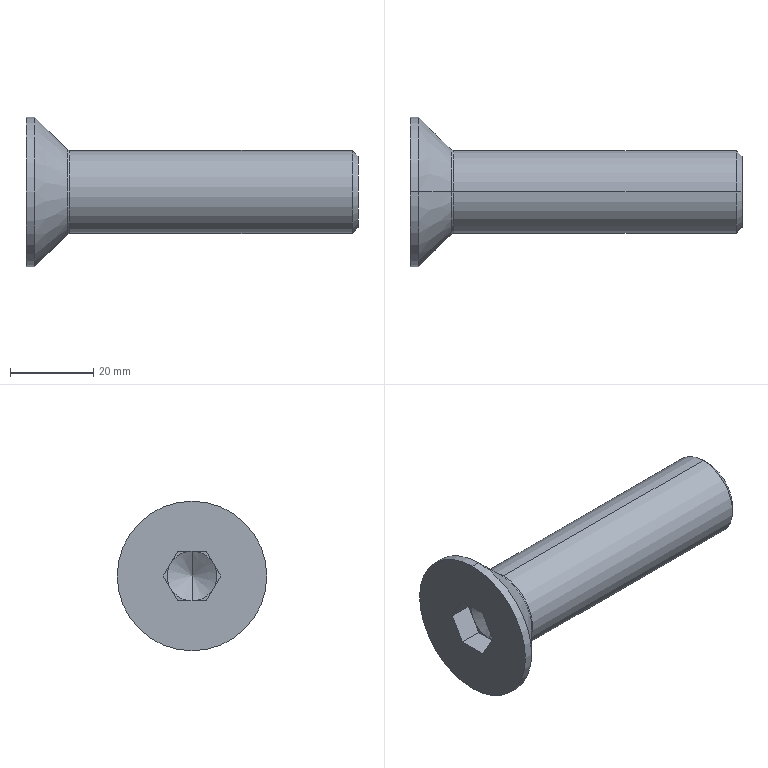Part | SolidWorks | features BaseBody 1 | 1 solid | 26 faces | box 80 x 36.05 x 36.05 mm | volume 28321 mm3 | plane 14 | cone 6 | cylinder 4 | spline 2 | commonest cylinder face diameters 20 x2 36.05 x2
STEP:
#1=CARTESIAN_POINT('',(10.491,0.,-10.));
#2=VERTEX_POINT('',#1);
#3=CARTESIAN_POINT('',(10.491,0.,10.));
#4=VERTEX_POINT('',#3);
#5=CARTESIAN_POINT('',(10.491,0.,0.));
#6=DIRECTION('',(1.,0.,0.));
#7=DIRECTION('',(0.,0.,1.));
#8=AXIS2_PLACEMENT_3D('',#5,#6,#7);
#9=CIRCLE('',#8,10.);
#10=EDGE_CURVE('',#2,#4,#9,.T.);
#11=ORIENTED_EDGE('',*,*,#10,.F.);
#12=CARTESIAN_POINT('',(9.926,0.,-10.234));
#13=VERTEX_POINT('',#12);
#14=CARTESIAN_POINT('',(10.491,0.,-10.8));
#15=DIRECTION('',(0.,-1.,0.));
#16=DIRECTION('',(0.,0.,-1.));
#17=AXIS2_PLACEMENT_3D('',#14,#15,#16);
#18=CIRCLE('',#17,0.8);
#19=EDGE_CURVE('',#2,#13,#18,.T.);
#20=ORIENTED_EDGE('',*,*,#19,.T.);
#21=CARTESIAN_POINT('',(9.926,0.,10.234));
#22=VERTEX_POINT('',#21);
#23=CARTESIAN_POINT('',(9.926,0.,0.));
#24=DIRECTION('',(-1.,0.,0.));
#25=DIRECTION('',(0.,0.,1.));
#26=AXIS2_PLACEMENT_3D('',#23,#24,#25);
#27=CIRCLE('',#26,10.234);
#28=EDGE_CURVE('',#22,#13,#27,.T.);
#29=ORIENTED_EDGE('',*,*,#28,.F.);
#30=CARTESIAN_POINT('',(10.491,0.,10.8));
#31=DIRECTION('',(0.,1.,0.));
#32=DIRECTION('',(0.,0.,1.));
#33=AXIS2_PLACEMENT_3D('',#30,#31,#32);
#34=CIRCLE('',#33,0.8);
#35=EDGE_CURVE('',#4,#22,#34,.T.);
#36=ORIENTED_EDGE('',*,*,#35,.F.);
#37=EDGE_LOOP('',(#11,#20,#29,#36));
#38=FACE_OUTER_BOUND('',#37,.T.);
#39=CARTESIAN_POINT('',(10.491,0.,10.));
#40=CARTESIAN_POINT('',(10.491,20.,10.));
#41=CARTESIAN_POINT('',(10.491,20.,-10.));
#42=CARTESIAN_POINT('',(10.491,0.,-10.));
#43=CARTESIAN_POINT('',(10.276,0.,10.));
#44=CARTESIAN_POINT('',(10.276,20.,10.));
#45=CARTESIAN_POINT('',(10.276,20.,-10.));
#46=CARTESIAN_POINT('',(10.276,0.,-10.));
#47=CARTESIAN_POINT('',(10.078,0.,10.082));
#48=CARTESIAN_POINT('',(10.078,20.165,10.082));
#49=CARTESIAN_POINT('',(10.078,20.165,-10.082));
#50=CARTESIAN_POINT('',(10.078,0.,-10.082));
#51=CARTESIAN_POINT('',(9.926,0.,10.234));
#52=CARTESIAN_POINT('',(9.926,20.469,10.234));
#53=CARTESIAN_POINT('',(9.926,20.469,-10.234));
#54=CARTESIAN_POINT('',(9.926,0.,-10.234));
#55=(BOUNDED_SURFACE()B_SPLINE_SURFACE(3,3,((#39,#40,#41,#42),(#43,#44,#45,#46),(#47,#48,#49,#50),(#51,#52,#53,#54)),.UNSPECIFIED.,.F.,.F.,.F.)B_SPLINE_SURFACE_WITH_KNOTS((4,4),(4,4),(0.,1.),(0.,1.),.UNSPECIFIED.)GEOMETRIC_REPRESENTATION_ITEM()RATIONAL_B_SPLINE_SURFACE(((1.,0.3333,0.3333,1.),(0.9493,0.3164,0.3164,0.9493),(0.9493,0.3164,0.3164,0.9493),(1.,0.3333,0.3333,1.)))REPRESENTATION_ITEM('')SURFACE());
#56=ADVANCED_FACE('',(#38),#55,.F.);
#57=CARTESIAN_POINT('',(78.626,0.,10.));
#58=VERTEX_POINT('',#57);
#59=CARTESIAN_POINT('',(78.626,0.,-10.));
#60=VERTEX_POINT('',#59);
#61=CARTESIAN_POINT('',(78.626,0.,0.));
#62=DIRECTION('',(-1.,0.,0.));
#63=DIRECTION('',(0.,0.,1.));
#64=AXIS2_PLACEMENT_3D('',#61,#62,#63);
#65=CIRCLE('',#64,10.);
#66=EDGE_CURVE('',#58,#60,#65,.T.);
#67=ORIENTED_EDGE('',*,*,#66,.T.);
#68=CARTESIAN_POINT('',(0.,0.,-10.));
#69=DIRECTION('',(-1.,0.,0.));
#70=VECTOR('',#69,1000.);
#71=LINE('',#68,#70);
#72=EDGE_CURVE('',#60,#2,#71,.T.);
#73=ORIENTED_EDGE('',*,*,#72,.T.);
#74=ORIENTED_EDGE('',*,*,#10,.T.);
#75=CARTESIAN_POINT('',(0.,0.,10.));
#76=DIRECTION('',(-1.,0.,0.));
#77=VECTOR('',#76,1000.);
#78=LINE('',#75,#77);
#79=EDGE_CURVE('',#58,#4,#78,.T.);
#80=ORIENTED_EDGE('',*,*,#79,.F.);
#81=EDGE_LOOP('',(#67,#73,#74,#80));
#82=FACE_OUTER_BOUND('',#81,.T.);
#83=CARTESIAN_POINT('',(0.,0.,0.));
#84=DIRECTION('',(-1.,0.,0.));
#85=DIRECTION('',(0.,0.,1.));
#86=AXIS2_PLACEMENT_3D('',#83,#84,#85);
#87=CYLINDRICAL_SURFACE('',#86,10.);
#88=ADVANCED_FACE('',(#82),#87,.T.);
#89=CARTESIAN_POINT('',(80.,0.,8.626));
#90=VERTEX_POINT('',#89);
#91=CARTESIAN_POINT('',(80.,0.,-8.626));
#92=VERTEX_POINT('',#91);
#93=CARTESIAN_POINT('',(80.,0.,0.));
#94=DIRECTION('',(-1.,0.,0.));
#95=DIRECTION('',(0.,0.,1.));
#96=AXIS2_PLACEMENT_3D('',#93,#94,#95);
#97=CIRCLE('',#96,8.626);
#98=EDGE_CURVE('',#90,#92,#97,.T.);
#99=ORIENTED_EDGE('',*,*,#98,.T.);
#100=CARTESIAN_POINT('',(78.626,0.,-10.));
#101=DIRECTION('',(-0.7071,0.,-0.7071));
#102=VECTOR('',#101,1000.);
#103=LINE('',#100,#102);
#104=EDGE_CURVE('',#92,#60,#103,.T.);
#105=ORIENTED_EDGE('',*,*,#104,.T.);
#106=ORIENTED_EDGE('',*,*,#66,.F.);
#107=CARTESIAN_POINT('',(78.626,0.,10.));
#108=DIRECTION('',(-0.7071,0.,0.7071));
#109=VECTOR('',#108,1000.);
#110=LINE('',#107,#109);
#111=EDGE_CURVE('',#90,#58,#110,.T.);
#112=ORIENTED_EDGE('',*,*,#111,.F.);
#113=EDGE_LOOP('',(#99,#105,#106,#112));
#114=FACE_OUTER_BOUND('',#113,.T.);
#115=CARTESIAN_POINT('',(78.626,0.,0.));
#116=DIRECTION('',(-1.,0.,0.));
#117=DIRECTION('',(0.,0.,1.));
#118=AXIS2_PLACEMENT_3D('',#115,#116,#117);
#119=CONICAL_SURFACE('',#118,10.,0.7854);
#120=ADVANCED_FACE('',(#114),#119,.T.);
#121=ORIENTED_EDGE('',*,*,#28,.T.);
#122=CARTESIAN_POINT('',(2.135,0.,-18.025));
#123=VERTEX_POINT('',#122);
#124=CARTESIAN_POINT('',(2.135,0.,-18.025));
#125=DIRECTION('',(-0.7071,0.,-0.7071));
#126=VECTOR('',#125,1000.);
#127=LINE('',#124,#126);
#128=EDGE_CURVE('',#13,#123,#127,.T.);
#129=ORIENTED_EDGE('',*,*,#128,.T.);
#130=CARTESIAN_POINT('',(2.135,0.,18.025));
#131=VERTEX_POINT('',#130);
#132=CARTESIAN_POINT('',(2.135,0.,0.));
#133=DIRECTION('',(1.,0.,0.));
#134=DIRECTION('',(0.,0.,1.));
#135=AXIS2_PLACEMENT_3D('',#132,#133,#134);
#136=CIRCLE('',#135,18.025);
#137=EDGE_CURVE('',#123,#131,#136,.T.);
#138=ORIENTED_EDGE('',*,*,#137,.T.);
#139=CARTESIAN_POINT('',(2.135,0.,18.025));
#140=DIRECTION('',(-0.7071,0.,0.7071));
#141=VECTOR('',#140,1000.);
#142=LINE('',#139,#141);
#143=EDGE_CURVE('',#22,#131,#142,.T.);
#144=ORIENTED_EDGE('',*,*,#143,.F.);
#145=EDGE_LOOP('',(#121,#129,#138,#144));
#146=FACE_OUTER_BOUND('',#145,.T.);
#147=CARTESIAN_POINT('',(2.135,0.,0.));
#148=DIRECTION('',(-1.,0.,0.));
#149=DIRECTION('',(0.,0.,1.));
#150=AXIS2_PLACEMENT_3D('',#147,#148,#149);
#151=CONICAL_SURFACE('',#150,18.025,0.7854);
#152=ADVANCED_FACE('',(#146),#151,.T.);
#153=ORIENTED_EDGE('',*,*,#137,.F.);
#154=CARTESIAN_POINT('',(0.,0.,-18.025));
#155=VERTEX_POINT('',#154);
#156=CARTESIAN_POINT('',(0.,0.,-18.025));
#157=DIRECTION('',(-1.,0.,0.));
#158=VECTOR('',#157,1000.);
#159=LINE('',#156,#158);
#160=EDGE_CURVE('',#123,#155,#159,.T.);
#161=ORIENTED_EDGE('',*,*,#160,.T.);
#162=CARTESIAN_POINT('',(0.,0.,18.025));
#163=VERTEX_POINT('',#162);
#164=CARTESIAN_POINT('',(0.,0.,0.));
#165=DIRECTION('',(1.,0.,0.));
#166=DIRECTION('',(0.,0.,1.));
#167=AXIS2_PLACEMENT_3D('',#164,#165,#166);
#168=CIRCLE('',#167,18.025);
#169=EDGE_CURVE('',#155,#163,#168,.T.);
#170=ORIENTED_EDGE('',*,*,#169,.T.);
#171=CARTESIAN_POINT('',(0.,0.,18.025));
#172=DIRECTION('',(-1.,0.,0.));
#173=VECTOR('',#172,1000.);
#174=LINE('',#171,#173);
#175=EDGE_CURVE('',#131,#163,#174,.T.);
#176=ORIENTED_EDGE('',*,*,#175,.F.);
#177=EDGE_LOOP('',(#153,#161,#170,#176));
#178=FACE_OUTER_BOUND('',#177,.T.);
#179=CARTESIAN_POINT('',(0.,0.,0.));
#180=DIRECTION('',(-1.,0.,0.));
#181=DIRECTION('',(0.,0.,1.));
#182=AXIS2_PLACEMENT_3D('',#179,#180,#181);
#183=CYLINDRICAL_SURFACE('',#182,18.025);
#184=ADVANCED_FACE('',(#178),#183,.T.);
#185=CARTESIAN_POINT('',(9.064,0.,0.));
#186=VERTEX_POINT('',#185);
#187=CARTESIAN_POINT('',(5.6,0.,6.));
#188=VERTEX_POINT('',#187);
#189=CARTESIAN_POINT('',(5.6,0.,6.));
#190=DIRECTION('',(-0.5,0.,0.866));
#191=VECTOR('',#190,1000.);
#192=LINE('',#189,#191);
#193=EDGE_CURVE('',#186,#188,#192,.T.);
#194=ORIENTED_EDGE('',*,*,#193,.F.);
#195=CARTESIAN_POINT('',(5.6,0.,-6.));
#196=VERTEX_POINT('',#195);
#197=CARTESIAN_POINT('',(5.6,0.,-6.));
#198=DIRECTION('',(-0.5,0.,-0.866));
#199=VECTOR('',#198,1000.);
#200=LINE('',#197,#199);
#201=EDGE_CURVE('',#186,#196,#200,.T.);
#202=ORIENTED_EDGE('',*,*,#201,.T.);
#203=CARTESIAN_POINT('',(5.6,-5.196,-3.));
#204=VERTEX_POINT('',#203);
#205=CARTESIAN_POINT('',(5.6,0.,0.));
#206=DIRECTION('',(-1.,0.,0.));
#207=DIRECTION('',(0.,0.,1.));
#208=AXIS2_PLACEMENT_3D('',#205,#206,#207);
#209=CIRCLE('',#208,6.);
#210=EDGE_CURVE('',#196,#204,#209,.T.);
#211=ORIENTED_EDGE('',*,*,#210,.T.);
#212=CARTESIAN_POINT('',(5.6,-5.196,3.));
#213=VERTEX_POINT('',#212);
#214=CARTESIAN_POINT('',(5.6,0.,0.));
#215=DIRECTION('',(-1.,0.,0.));
#216=DIRECTION('',(0.,0.,1.));
#217=AXIS2_PLACEMENT_3D('',#214,#215,#216);
#218=CIRCLE('',#217,6.);
#219=EDGE_CURVE('',#204,#213,#218,.T.);
#220=ORIENTED_EDGE('',*,*,#219,.T.);
#221=CARTESIAN_POINT('',(5.6,0.,0.));
#222=DIRECTION('',(-1.,0.,0.));
#223=DIRECTION('',(0.,0.,1.));
#224=AXIS2_PLACEMENT_3D('',#221,#222,#223);
#225=CIRCLE('',#224,6.);
#226=EDGE_CURVE('',#213,#188,#225,.T.);
#227=ORIENTED_EDGE('',*,*,#226,.T.);
#228=EDGE_LOOP('',(#194,#202,#211,#220,#227));
#229=FACE_OUTER_BOUND('',#228,.T.);
#230=CARTESIAN_POINT('',(5.6,0.,0.));
#231=DIRECTION('',(-1.,0.,0.));
#232=DIRECTION('',(0.,0.,1.));
#233=AXIS2_PLACEMENT_3D('',#230,#231,#232);
#234=CONICAL_SURFACE('',#233,6.,1.047);
#235=ADVANCED_FACE('',(#229),#234,.F.);
#236=ORIENTED_EDGE('',*,*,#72,.F.);
#237=CARTESIAN_POINT('',(78.626,0.,0.));
#238=DIRECTION('',(-1.,0.,0.));
#239=DIRECTION('',(0.,0.,1.));
#240=AXIS2_PLACEMENT_3D('',#237,#238,#239);
#241=CIRCLE('',#240,10.);
#242=EDGE_CURVE('',#60,#58,#241,.T.);
#243=ORIENTED_EDGE('',*,*,#242,.T.);
#244=ORIENTED_EDGE('',*,*,#79,.T.);
#245=CARTESIAN_POINT('',(10.491,0.,0.));
#246=DIRECTION('',(1.,0.,0.));
#247=DIRECTION('',(0.,0.,1.));
#248=AXIS2_PLACEMENT_3D('',#245,#246,#247);
#249=CIRCLE('',#248,10.);
#250=EDGE_CURVE('',#4,#2,#249,.T.);
#251=ORIENTED_EDGE('',*,*,#250,.T.);
#252=EDGE_LOOP('',(#236,#243,#244,#251));
#253=FACE_OUTER_BOUND('',#252,.T.);
#254=CARTESIAN_POINT('',(0.,0.,0.));
#255=DIRECTION('',(-1.,0.,0.));
#256=DIRECTION('',(0.,0.,1.));
#257=AXIS2_PLACEMENT_3D('',#254,#255,#256);
#258=CYLINDRICAL_SURFACE('',#257,10.);
#259=ADVANCED_FACE('',(#253),#258,.T.);
#260=ORIENTED_EDGE('',*,*,#19,.F.);
#261=ORIENTED_EDGE('',*,*,#250,.F.);
#262=ORIENTED_EDGE('',*,*,#35,.T.);
#263=CARTESIAN_POINT('',(9.926,0.,0.));
#264=DIRECTION('',(-1.,0.,0.));
#265=DIRECTION('',(0.,0.,1.));
#266=AXIS2_PLACEMENT_3D('',#263,#264,#265);
#267=CIRCLE('',#266,10.234);
#268=EDGE_CURVE('',#13,#22,#267,.T.);
#269=ORIENTED_EDGE('',*,*,#268,.F.);
#270=EDGE_LOOP('',(#260,#261,#262,#269));
#271=FACE_OUTER_BOUND('',#270,.T.);
#272=CARTESIAN_POINT('',(10.491,0.,-10.));
#273=CARTESIAN_POINT('',(10.491,-20.,-10.));
#274=CARTESIAN_POINT('',(10.491,-20.,10.));
#275=CARTESIAN_POINT('',(10.491,0.,10.));
#276=CARTESIAN_POINT('',(10.276,0.,-10.));
#277=CARTESIAN_POINT('',(10.276,-20.,-10.));
#278=CARTESIAN_POINT('',(10.276,-20.,10.));
#279=CARTESIAN_POINT('',(10.276,0.,10.));
#280=CARTESIAN_POINT('',(10.078,0.,-10.082));
#281=CARTESIAN_POINT('',(10.078,-20.165,-10.082));
#282=CARTESIAN_POINT('',(10.078,-20.165,10.082));
#283=CARTESIAN_POINT('',(10.078,0.,10.082));
#284=CARTESIAN_POINT('',(9.926,0.,-10.234));
#285=CARTESIAN_POINT('',(9.926,-20.469,-10.234));
#286=CARTESIAN_POINT('',(9.926,-20.469,10.234));
#287=CARTESIAN_POINT('',(9.926,0.,10.234));
#288=(BOUNDED_SURFACE()B_SPLINE_SURFACE(3,3,((#272,#273,#274,#275),(#276,#277,#278,#279),(#280,#281,#282,#283),(#284,#285,#286,#287)),.UNSPECIFIED.,.F.,.F.,.F.)B_SPLINE_SURFACE_WITH_KNOTS((4,4),(4,4),(0.,1.),(0.,1.),.UNSPECIFIED.)GEOMETRIC_REPRESENTATION_ITEM()RATIONAL_B_SPLINE_SURFACE(((1.,0.3333,0.3333,1.),(0.9493,0.3164,0.3164,0.9493),(0.9493,0.3164,0.3164,0.9493),(1.,0.3333,0.3333,1.)))REPRESENTATION_ITEM('')SURFACE());
#289=ADVANCED_FACE('',(#271),#288,.F.);
#290=ORIENTED_EDGE('',*,*,#104,.F.);
#291=CARTESIAN_POINT('',(80.,0.,0.));
#292=DIRECTION('',(-1.,0.,0.));
#293=DIRECTION('',(0.,0.,1.));
#294=AXIS2_PLACEMENT_3D('',#291,#292,#293);
#295=CIRCLE('',#294,8.626);
#296=EDGE_CURVE('',#92,#90,#295,.T.);
#297=ORIENTED_EDGE('',*,*,#296,.T.);
#298=ORIENTED_EDGE('',*,*,#111,.T.);
#299=ORIENTED_EDGE('',*,*,#242,.F.);
#300=EDGE_LOOP('',(#290,#297,#298,#299));
#301=FACE_OUTER_BOUND('',#300,.T.);
#302=CARTESIAN_POINT('',(78.626,0.,0.));
#303=DIRECTION('',(-1.,0.,0.));
#304=DIRECTION('',(0.,0.,1.));
#305=AXIS2_PLACEMENT_3D('',#302,#303,#304);
#306=CONICAL_SURFACE('',#305,10.,0.7854);
#307=ADVANCED_FACE('',(#301),#306,.T.);
#308=ORIENTED_EDGE('',*,*,#128,.F.);
#309=ORIENTED_EDGE('',*,*,#268,.T.);
#310=ORIENTED_EDGE('',*,*,#143,.T.);
#311=CARTESIAN_POINT('',(2.135,0.,0.));
#312=DIRECTION('',(1.,0.,0.));
#313=DIRECTION('',(0.,0.,1.));
#314=AXIS2_PLACEMENT_3D('',#311,#312,#313);
#315=CIRCLE('',#314,18.025);
#316=EDGE_CURVE('',#131,#123,#315,.T.);
#317=ORIENTED_EDGE('',*,*,#316,.T.);
#318=EDGE_LOOP('',(#308,#309,#310,#317));
#319=FACE_OUTER_BOUND('',#318,.T.);
#320=CARTESIAN_POINT('',(2.135,0.,0.));
#321=DIRECTION('',(-1.,0.,0.));
#322=DIRECTION('',(0.,0.,1.));
#323=AXIS2_PLACEMENT_3D('',#320,#321,#322);
#324=CONICAL_SURFACE('',#323,18.025,0.7854);
#325=ADVANCED_FACE('',(#319),#324,.T.);
#326=ORIENTED_EDGE('',*,*,#98,.F.);
#327=ORIENTED_EDGE('',*,*,#296,.F.);
#328=EDGE_LOOP('',(#326,#327));
#329=FACE_OUTER_BOUND('',#328,.T.);
#330=CARTESIAN_POINT('',(80.,8.626,0.));
#331=DIRECTION('',(1.,0.,0.));
#332=DIRECTION('',(0.,0.,-1.));
#333=AXIS2_PLACEMENT_3D('',#330,#331,#332);
#334=PLANE('',#333);
#335=ADVANCED_FACE('',(#329),#334,.T.);
#336=ORIENTED_EDGE('',*,*,#160,.F.);
#337=ORIENTED_EDGE('',*,*,#316,.F.);
#338=ORIENTED_EDGE('',*,*,#175,.T.);
#339=CARTESIAN_POINT('',(0.,0.,0.));
#340=DIRECTION('',(1.,0.,0.));
#341=DIRECTION('',(0.,0.,1.));
#342=AXIS2_PLACEMENT_3D('',#339,#340,#341);
#343=CIRCLE('',#342,18.025);
#344=EDGE_CURVE('',#163,#155,#343,.T.);
#345=ORIENTED_EDGE('',*,*,#344,.T.);
#346=EDGE_LOOP('',(#336,#337,#338,#345));
#347=FACE_OUTER_BOUND('',#346,.T.);
#348=CARTESIAN_POINT('',(0.,0.,0.));
#349=DIRECTION('',(-1.,0.,0.));
#350=DIRECTION('',(0.,0.,1.));
#351=AXIS2_PLACEMENT_3D('',#348,#349,#350);
#352=CYLINDRICAL_SURFACE('',#351,18.025);
#353=ADVANCED_FACE('',(#347),#352,.T.);
#354=CARTESIAN_POINT('',(0.,6.928,0.));
#355=VERTEX_POINT('',#354);
#356=CARTESIAN_POINT('',(0.,3.464,6.));
#357=VERTEX_POINT('',#356);
#358=CARTESIAN_POINT('',(0.,6.928,0.));
#359=DIRECTION('',(0.,-0.5,0.866));
#360=VECTOR('',#359,1000.);
#361=LINE('',#358,#360);
#362=EDGE_CURVE('',#355,#357,#361,.T.);
#363=ORIENTED_EDGE('',*,*,#362,.T.);
#364=CARTESIAN_POINT('',(0.,-3.464,6.));
#365=VERTEX_POINT('',#364);
#366=CARTESIAN_POINT('',(0.,0.,6.));
#367=DIRECTION('',(0.,-1.,0.));
#368=VECTOR('',#367,1000.);
#369=LINE('',#366,#368);
#370=EDGE_CURVE('',#357,#365,#369,.T.);
#371=ORIENTED_EDGE('',*,*,#370,.T.);
#372=CARTESIAN_POINT('',(0.,-6.928,0.));
#373=VERTEX_POINT('',#372);
#374=CARTESIAN_POINT('',(0.,-3.464,6.));
#375=DIRECTION('',(0.,-0.5,-0.866));
#376=VECTOR('',#375,1000.);
#377=LINE('',#374,#376);
#378=EDGE_CURVE('',#365,#373,#377,.T.);
#379=ORIENTED_EDGE('',*,*,#378,.T.);
#380=CARTESIAN_POINT('',(0.,-3.464,-6.));
#381=VERTEX_POINT('',#380);
#382=CARTESIAN_POINT('',(0.,-6.928,0.));
#383=DIRECTION('',(0.,0.5,-0.866));
#384=VECTOR('',#383,1000.);
#385=LINE('',#382,#384);
#386=EDGE_CURVE('',#373,#381,#385,.T.);
#387=ORIENTED_EDGE('',*,*,#386,.T.);
#388=CARTESIAN_POINT('',(0.,3.464,-6.));
#389=VERTEX_POINT('',#388);
#390=CARTESIAN_POINT('',(0.,0.,-6.));
#391=DIRECTION('',(0.,1.,0.));
#392=VECTOR('',#391,1000.);
#393=LINE('',#390,#392);
#394=EDGE_CURVE('',#381,#389,#393,.T.);
#395=ORIENTED_EDGE('',*,*,#394,.T.);
#396=CARTESIAN_POINT('',(0.,3.464,-6.));
#397=DIRECTION('',(0.,0.5,0.866));
#398=VECTOR('',#397,1000.);
#399=LINE('',#396,#398);
#400=EDGE_CURVE('',#389,#355,#399,.T.);
#401=ORIENTED_EDGE('',*,*,#400,.T.);
#402=EDGE_LOOP('',(#363,#371,#379,#387,#395,#401));
#403=FACE_BOUND('',#402,.T.);
#404=ORIENTED_EDGE('',*,*,#344,.F.);
#405=ORIENTED_EDGE('',*,*,#169,.F.);
#406=EDGE_LOOP('',(#404,#405));
#407=FACE_OUTER_BOUND('',#406,.T.);
#408=CARTESIAN_POINT('',(0.,0.,0.));
#409=DIRECTION('',(-1.,0.,0.));
#410=DIRECTION('',(0.,0.,1.));
#411=AXIS2_PLACEMENT_3D('',#408,#409,#410);
#412=PLANE('',#411);
#413=ADVANCED_FACE('',(#403,#407),#412,.T.);
#414=CARTESIAN_POINT('',(5.6,-3.464,6.));
#415=VERTEX_POINT('',#414);
#416=CARTESIAN_POINT('',(5.6,3.464,6.));
#417=DIRECTION('',(0.,-1.,0.));
#418=VECTOR('',#417,1000.);
#419=LINE('',#416,#418);
#420=EDGE_CURVE('',#188,#415,#419,.T.);
#421=ORIENTED_EDGE('',*,*,#420,.T.);
#422=CARTESIAN_POINT('',(5.6,-3.464,6.));
#423=DIRECTION('',(-1.,0.,0.));
#424=VECTOR('',#423,1000.);
#425=LINE('',#422,#424);
#426=EDGE_CURVE('',#415,#365,#425,.T.);
#427=ORIENTED_EDGE('',*,*,#426,.T.);
#428=ORIENTED_EDGE('',*,*,#370,.F.);
#429=CARTESIAN_POINT('',(5.6,3.464,6.));
#430=VERTEX_POINT('',#429);
#431=CARTESIAN_POINT('',(5.6,3.464,6.));
#432=DIRECTION('',(1.,0.,0.));
#433=VECTOR('',#432,1000.);
#434=LINE('',#431,#433);
#435=EDGE_CURVE('',#357,#430,#434,.T.);
#436=ORIENTED_EDGE('',*,*,#435,.T.);
#437=CARTESIAN_POINT('',(5.6,3.464,6.));
#438=DIRECTION('',(0.,-1.,0.));
#439=VECTOR('',#438,1000.);
#440=LINE('',#437,#439);
#441=EDGE_CURVE('',#430,#188,#440,.T.);
#442=ORIENTED_EDGE('',*,*,#441,.T.);
#443=EDGE_LOOP('',(#421,#427,#428,#436,#442));
#444=FACE_OUTER_BOUND('',#443,.T.);
#445=CARTESIAN_POINT('',(5.6,3.464,6.));
#446=DIRECTION('',(0.,0.,-1.));
#447=DIRECTION('',(-1.,0.,0.));
#448=AXIS2_PLACEMENT_3D('',#445,#446,#447);
#449=PLANE('',#448);
#450=ADVANCED_FACE('',(#444),#449,.T.);
#451=CARTESIAN_POINT('',(5.6,5.196,3.));
#452=VERTEX_POINT('',#451);
#453=CARTESIAN_POINT('',(5.6,6.928,0.));
#454=DIRECTION('',(0.,-0.5,0.866));
#455=VECTOR('',#454,1000.);
#456=LINE('',#453,#455);
#457=EDGE_CURVE('',#452,#430,#456,.T.);
#458=ORIENTED_EDGE('',*,*,#457,.T.);
#459=ORIENTED_EDGE('',*,*,#435,.F.);
#460=ORIENTED_EDGE('',*,*,#362,.F.);
#461=CARTESIAN_POINT('',(5.6,6.928,0.));
#462=VERTEX_POINT('',#461);
#463=CARTESIAN_POINT('',(5.6,6.928,0.));
#464=DIRECTION('',(1.,0.,0.));
#465=VECTOR('',#464,1000.);
#466=LINE('',#463,#465);
#467=EDGE_CURVE('',#355,#462,#466,.T.);
#468=ORIENTED_EDGE('',*,*,#467,.T.);
#469=CARTESIAN_POINT('',(5.6,6.928,0.));
#470=DIRECTION('',(0.,-0.5,0.866));
#471=VECTOR('',#470,1000.);
#472=LINE('',#469,#471);
#473=EDGE_CURVE('',#462,#452,#472,.T.);
#474=ORIENTED_EDGE('',*,*,#473,.T.);
#475=EDGE_LOOP('',(#458,#459,#460,#468,#474));
#476=FACE_OUTER_BOUND('',#475,.T.);
#477=CARTESIAN_POINT('',(5.6,6.928,0.));
#478=DIRECTION('',(0.,-0.866,-0.5));
#479=DIRECTION('',(0.,0.5,-0.866));
#480=AXIS2_PLACEMENT_3D('',#477,#478,#479);
#481=PLANE('',#480);
#482=ADVANCED_FACE('',(#476),#481,.T.);
#483=CARTESIAN_POINT('',(5.6,5.196,-3.));
#484=VERTEX_POINT('',#483);
#485=CARTESIAN_POINT('',(5.6,3.464,-6.));
#486=DIRECTION('',(0.,0.5,0.866));
#487=VECTOR('',#486,1000.);
#488=LINE('',#485,#487);
#489=EDGE_CURVE('',#484,#462,#488,.T.);
#490=ORIENTED_EDGE('',*,*,#489,.T.);
#491=ORIENTED_EDGE('',*,*,#467,.F.);
#492=ORIENTED_EDGE('',*,*,#400,.F.);
#493=CARTESIAN_POINT('',(5.6,3.464,-6.));
#494=VERTEX_POINT('',#493);
#495=CARTESIAN_POINT('',(5.6,3.464,-6.));
#496=DIRECTION('',(1.,0.,0.));
#497=VECTOR('',#496,1000.);
#498=LINE('',#495,#497);
#499=EDGE_CURVE('',#389,#494,#498,.T.);
#500=ORIENTED_EDGE('',*,*,#499,.T.);
#501=CARTESIAN_POINT('',(5.6,3.464,-6.));
#502=DIRECTION('',(0.,0.5,0.866));
#503=VECTOR('',#502,1000.);
#504=LINE('',#501,#503);
#505=EDGE_CURVE('',#494,#484,#504,.T.);
#506=ORIENTED_EDGE('',*,*,#505,.T.);
#507=EDGE_LOOP('',(#490,#491,#492,#500,#506));
#508=FACE_OUTER_BOUND('',#507,.T.);
#509=CARTESIAN_POINT('',(5.6,3.464,-6.));
#510=DIRECTION('',(0.,-0.866,0.5));
#511=DIRECTION('',(0.,-0.5,-0.866));
#512=AXIS2_PLACEMENT_3D('',#509,#510,#511);
#513=PLANE('',#512);
#514=ADVANCED_FACE('',(#508),#513,.T.);
#515=CARTESIAN_POINT('',(5.6,-3.464,-6.));
#516=DIRECTION('',(0.,1.,0.));
#517=VECTOR('',#516,1000.);
#518=LINE('',#515,#517);
#519=EDGE_CURVE('',#196,#494,#518,.T.);
#520=ORIENTED_EDGE('',*,*,#519,.T.);
#521=ORIENTED_EDGE('',*,*,#499,.F.);
#522=ORIENTED_EDGE('',*,*,#394,.F.);
#523=CARTESIAN_POINT('',(5.6,-3.464,-6.));
#524=VERTEX_POINT('',#523);
#525=CARTESIAN_POINT('',(5.6,-3.464,-6.));
#526=DIRECTION('',(1.,0.,0.));
#527=VECTOR('',#526,1000.);
#528=LINE('',#525,#527);
#529=EDGE_CURVE('',#381,#524,#528,.T.);
#530=ORIENTED_EDGE('',*,*,#529,.T.);
#531=CARTESIAN_POINT('',(5.6,-3.464,-6.));
#532=DIRECTION('',(0.,1.,0.));
#533=VECTOR('',#532,1000.);
#534=LINE('',#531,#533);
#535=EDGE_CURVE('',#524,#196,#534,.T.);
#536=ORIENTED_EDGE('',*,*,#535,.T.);
#537=EDGE_LOOP('',(#520,#521,#522,#530,#536));
#538=FACE_OUTER_BOUND('',#537,.T.);
#539=CARTESIAN_POINT('',(5.6,-3.464,-6.));
#540=DIRECTION('',(0.,0.,1.));
#541=DIRECTION('',(0.,-1.,0.));
#542=AXIS2_PLACEMENT_3D('',#539,#540,#541);
#543=PLANE('',#542);
#544=ADVANCED_FACE('',(#538),#543,.T.);
#545=CARTESIAN_POINT('',(5.6,-6.928,0.));
#546=DIRECTION('',(0.,0.5,-0.866));
#547=VECTOR('',#546,1000.);
#548=LINE('',#545,#547);
#549=EDGE_CURVE('',#204,#524,#548,.T.);
#550=ORIENTED_EDGE('',*,*,#549,.T.);
#551=ORIENTED_EDGE('',*,*,#529,.F.);
#552=ORIENTED_EDGE('',*,*,#386,.F.);
#553=CARTESIAN_POINT('',(5.6,-6.928,0.));
#554=VERTEX_POINT('',#553);
#555=CARTESIAN_POINT('',(5.6,-6.928,0.));
#556=DIRECTION('',(1.,0.,0.));
#557=VECTOR('',#556,1000.);
#558=LINE('',#555,#557);
#559=EDGE_CURVE('',#373,#554,#558,.T.);
#560=ORIENTED_EDGE('',*,*,#559,.T.);
#561=CARTESIAN_POINT('',(5.6,-6.928,0.));
#562=DIRECTION('',(0.,0.5,-0.866));
#563=VECTOR('',#562,1000.);
#564=LINE('',#561,#563);
#565=EDGE_CURVE('',#554,#204,#564,.T.);
#566=ORIENTED_EDGE('',*,*,#565,.T.);
#567=EDGE_LOOP('',(#550,#551,#552,#560,#566));
#568=FACE_OUTER_BOUND('',#567,.T.);
#569=CARTESIAN_POINT('',(5.6,-6.928,0.));
#570=DIRECTION('',(0.,0.866,0.5));
#571=DIRECTION('',(0.,-0.5,0.866));
#572=AXIS2_PLACEMENT_3D('',#569,#570,#571);
#573=PLANE('',#572);
#574=ADVANCED_FACE('',(#568),#573,.T.);
#575=CARTESIAN_POINT('',(5.6,-3.464,6.));
#576=DIRECTION('',(0.,-0.5,-0.866));
#577=VECTOR('',#576,1000.);
#578=LINE('',#575,#577);
#579=EDGE_CURVE('',#213,#554,#578,.T.);
#580=ORIENTED_EDGE('',*,*,#579,.T.);
#581=ORIENTED_EDGE('',*,*,#559,.F.);
#582=ORIENTED_EDGE('',*,*,#378,.F.);
#583=ORIENTED_EDGE('',*,*,#426,.F.);
#584=CARTESIAN_POINT('',(5.6,-3.464,6.));
#585=DIRECTION('',(0.,-0.5,-0.866));
#586=VECTOR('',#585,1000.);
#587=LINE('',#584,#586);
#588=EDGE_CURVE('',#415,#213,#587,.T.);
#589=ORIENTED_EDGE('',*,*,#588,.T.);
#590=EDGE_LOOP('',(#580,#581,#582,#583,#589));
#591=FACE_OUTER_BOUND('',#590,.T.);
#592=CARTESIAN_POINT('',(5.6,-3.464,6.));
#593=DIRECTION('',(0.,0.866,-0.5));
#594=DIRECTION('',(0.,0.5,0.866));
#595=AXIS2_PLACEMENT_3D('',#592,#593,#594);
#596=PLANE('',#595);
#597=ADVANCED_FACE('',(#591),#596,.T.);
#598=ORIENTED_EDGE('',*,*,#420,.F.);
#599=ORIENTED_EDGE('',*,*,#226,.F.);
#600=ORIENTED_EDGE('',*,*,#588,.F.);
#601=EDGE_LOOP('',(#598,#599,#600));
#602=FACE_OUTER_BOUND('',#601,.T.);
#603=CARTESIAN_POINT('',(5.6,-3.464,-6.));
#604=DIRECTION('',(1.,0.,0.));
#605=DIRECTION('',(0.,0.,-1.));
#606=AXIS2_PLACEMENT_3D('',#603,#604,#605);
#607=PLANE('',#606);
#608=ADVANCED_FACE('',(#602),#607,.F.);
#609=ORIENTED_EDGE('',*,*,#457,.F.);
#610=CARTESIAN_POINT('',(5.6,0.,0.));
#611=DIRECTION('',(-1.,0.,0.));
#612=DIRECTION('',(0.,0.,1.));
#613=AXIS2_PLACEMENT_3D('',#610,#611,#612);
#614=CIRCLE('',#613,6.);
#615=EDGE_CURVE('',#188,#452,#614,.T.);
#616=ORIENTED_EDGE('',*,*,#615,.F.);
#617=ORIENTED_EDGE('',*,*,#441,.F.);
#618=EDGE_LOOP('',(#609,#616,#617));
#619=FACE_OUTER_BOUND('',#618,.T.);
#620=CARTESIAN_POINT('',(5.6,-3.464,-6.));
#621=DIRECTION('',(1.,0.,0.));
#622=DIRECTION('',(0.,0.,-1.));
#623=AXIS2_PLACEMENT_3D('',#620,#621,#622);
#624=PLANE('',#623);
#625=ADVANCED_FACE('',(#619),#624,.F.);
#626=ORIENTED_EDGE('',*,*,#489,.F.);
#627=CARTESIAN_POINT('',(5.6,0.,0.));
#628=DIRECTION('',(-1.,0.,0.));
#629=DIRECTION('',(0.,0.,1.));
#630=AXIS2_PLACEMENT_3D('',#627,#628,#629);
#631=CIRCLE('',#630,6.);
#632=EDGE_CURVE('',#452,#484,#631,.T.);
#633=ORIENTED_EDGE('',*,*,#632,.F.);
#634=ORIENTED_EDGE('',*,*,#473,.F.);
#635=EDGE_LOOP('',(#626,#633,#634));
#636=FACE_OUTER_BOUND('',#635,.T.);
#637=CARTESIAN_POINT('',(5.6,-3.464,-6.));
#638=DIRECTION('',(1.,0.,0.));
#639=DIRECTION('',(0.,0.,-1.));
#640=AXIS2_PLACEMENT_3D('',#637,#638,#639);
#641=PLANE('',#640);
#642=ADVANCED_FACE('',(#636),#641,.F.);
#643=ORIENTED_EDGE('',*,*,#519,.F.);
#644=CARTESIAN_POINT('',(5.6,0.,0.));
#645=DIRECTION('',(-1.,0.,0.));
#646=DIRECTION('',(0.,0.,1.));
#647=AXIS2_PLACEMENT_3D('',#644,#645,#646);
#648=CIRCLE('',#647,6.);
#649=EDGE_CURVE('',#484,#196,#648,.T.);
#650=ORIENTED_EDGE('',*,*,#649,.F.);
#651=ORIENTED_EDGE('',*,*,#505,.F.);
#652=EDGE_LOOP('',(#643,#650,#651));
#653=FACE_OUTER_BOUND('',#652,.T.);
#654=CARTESIAN_POINT('',(5.6,-3.464,-6.));
#655=DIRECTION('',(1.,0.,0.));
#656=DIRECTION('',(0.,0.,-1.));
#657=AXIS2_PLACEMENT_3D('',#654,#655,#656);
#658=PLANE('',#657);
#659=ADVANCED_FACE('',(#653),#658,.F.);
#660=ORIENTED_EDGE('',*,*,#549,.F.);
#661=ORIENTED_EDGE('',*,*,#210,.F.);
#662=ORIENTED_EDGE('',*,*,#535,.F.);
#663=EDGE_LOOP('',(#660,#661,#662));
#664=FACE_OUTER_BOUND('',#663,.T.);
#665=CARTESIAN_POINT('',(5.6,-3.464,-6.));
#666=DIRECTION('',(1.,0.,0.));
#667=DIRECTION('',(0.,0.,-1.));
#668=AXIS2_PLACEMENT_3D('',#665,#666,#667);
#669=PLANE('',#668);
#670=ADVANCED_FACE('',(#664),#669,.F.);
#671=ORIENTED_EDGE('',*,*,#579,.F.);
#672=ORIENTED_EDGE('',*,*,#219,.F.);
#673=ORIENTED_EDGE('',*,*,#565,.F.);
#674=EDGE_LOOP('',(#671,#672,#673));
#675=FACE_OUTER_BOUND('',#674,.T.);
#676=CARTESIAN_POINT('',(5.6,-3.464,-6.));
#677=DIRECTION('',(1.,0.,0.));
#678=DIRECTION('',(0.,0.,-1.));
#679=AXIS2_PLACEMENT_3D('',#676,#677,#678);
#680=PLANE('',#679);
#681=ADVANCED_FACE('',(#675),#680,.F.);
#682=ORIENTED_EDGE('',*,*,#201,.F.);
#683=ORIENTED_EDGE('',*,*,#193,.T.);
#684=ORIENTED_EDGE('',*,*,#615,.T.);
#685=ORIENTED_EDGE('',*,*,#632,.T.);
#686=ORIENTED_EDGE('',*,*,#649,.T.);
#687=EDGE_LOOP('',(#682,#683,#684,#685,#686));
#688=FACE_OUTER_BOUND('',#687,.T.);
#689=CARTESIAN_POINT('',(5.6,0.,0.));
#690=DIRECTION('',(-1.,0.,0.));
#691=DIRECTION('',(0.,0.,1.));
#692=AXIS2_PLACEMENT_3D('',#689,#690,#691);
#693=CONICAL_SURFACE('',#692,6.,1.047);
#694=ADVANCED_FACE('',(#688),#693,.F.);
#695=CLOSED_SHELL('',(#56,#88,#120,#152,#184,#235,#259,#289,#307,#325,#335,#353,#413,#450,#482,#514,#544,#574,#597,#608,#625,#642,#659,#670,#681,#694));
#696=MANIFOLD_SOLID_BREP('',#695);
#697=CARTESIAN_POINT('',(0.,0.,0.));
#698=DIRECTION('',(0.,0.,1.));
#699=DIRECTION('',(1.,0.,0.));
#700=AXIS2_PLACEMENT_3D('',#697,#698,#699);
#701=(LENGTH_UNIT()NAMED_UNIT(*)SI_UNIT(.MILLI.,.METRE.));
#702=UNCERTAINTY_MEASURE_WITH_UNIT(LENGTH_MEASURE(0.00001),#701,'','');
#703=(NAMED_UNIT(*)PLANE_ANGLE_UNIT()SI_UNIT($,.RADIAN.));
#704=(NAMED_UNIT(*)SI_UNIT($,.STERADIAN.)SOLID_ANGLE_UNIT());
#705=(GEOMETRIC_REPRESENTATION_CONTEXT(3)GLOBAL_UNCERTAINTY_ASSIGNED_CONTEXT((#702))GLOBAL_UNIT_ASSIGNED_CONTEXT((#701,#703,#704))REPRESENTATION_CONTEXT('',''));
#706=ADVANCED_BREP_SHAPE_REPRESENTATION('',(#696,#700),#705);